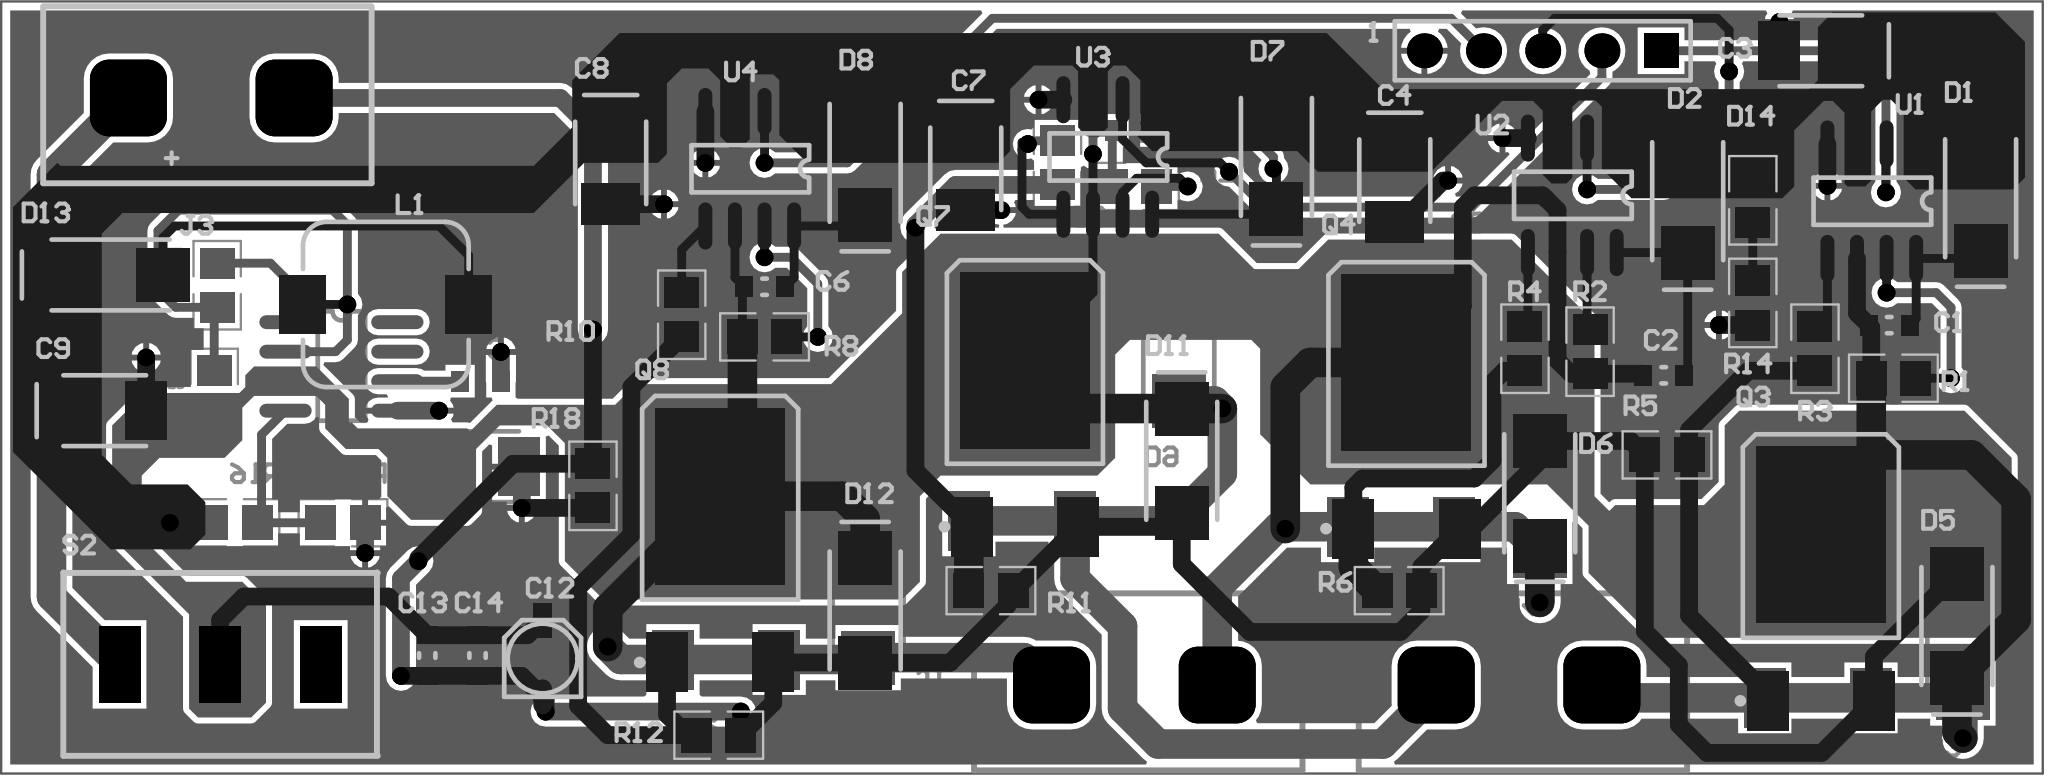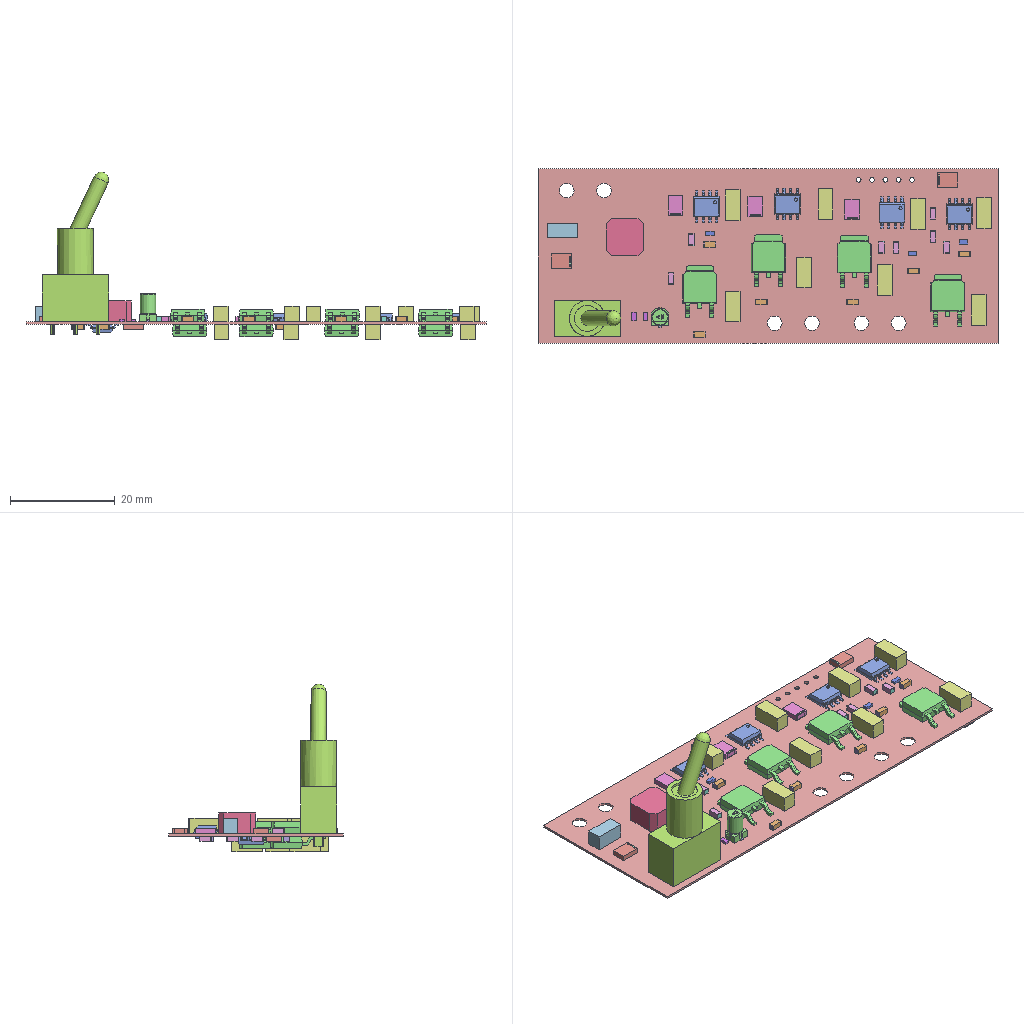Circuit board layout | Altium Designer | box 87.6 x 33.2 x 32 mm
Layer stack:
# Altium Designer layer stack of  (unit mm; dielectric type: 0 none, 1 core, 2 prepreg, 3 surface material)
index,name,kind,layer,copper_thickness_mm,dielectric_type,dielectric_thickness_mm,dielectric_material,dielectric_constant
0,Top Paste,other,,,,,,
1,Top Overlay,other,,,,,,
2,Top Solder,dielectric,,,3,0.0102,Solder Resist,3.5
3,Top Layer,copper,Top Layer,0.0356,,,,
4,Dielectric 1,dielectric,,,0,0.32,FR-4,4.8
5,Bottom Layer,copper,Bottom Layer,0.0356,,,,
6,Bottom Solder,dielectric,,,3,0.0102,Solder Resist,3.5
7,Bottom Overlay,other,,,,,,
8,Bottom Paste,other,,,,,,
# drill layer pairs: low layer,high layer
drill_pair,Top Layer,Bottom Layer
Part placement:
Designator,Comment,Layer,Footprint,Center-X(mm),Center-Y(mm),Rotation
U5,MC34063,BottomLayer,MC34063,33.782,84.455,180
U4,IR2104S,TopLayer,IR2104,51.308,92.964,270
U3,IR2104S,TopLayer,IR2104,66.675,93.472,270
U2,IR2104S,TopLayer,IR2104,86.614,91.821,270
U1,IR2104S,TopLayer,IR2104,99.469,91.567,270
S2,SW-SPST,TopLayer,SWITCH,28.575,71.628,360
R18,Res1,TopLayer,0805,44.577,79.314,270
R17,Res1,BottomLayer,0805,33.848,77.724,360
R16,Res1,BottomLayer,0805,29.21,77.724,360
R15,Res1,BottomLayer,0805,28.448,87.95,270
R14,Res1,TopLayer,0805,94.361,87.188,270
R13,Res1,BottomLayer,0805,28.321,83.312,270
R12,Res1,TopLayer,0805,49.977,68.58,180
R11,Res1,TopLayer,0805,61.661,74.803,180
R10,Res1,TopLayer,0805,48.387,86.68,270
R9,Res1,BottomLayer,0805,64.516,93.218,270
R8,Res1,TopLayer,0805,51.943,85.725,180
R7,Res1,BottomLayer,0805,67.818,92.202,180
R6,Res1,TopLayer,0805,79.182,74.803,180
R5,Res1,TopLayer,0805,90.678,80.645,360
R4,Res1,TopLayer,0805,84.582,85.217,270
R3,Res1,TopLayer,0805,97.028,85.217,270
R2,Res1,TopLayer,0805,87.376,85.09,270
R1,Res1,TopLayer,0805,100.396,83.947,180
Q8,IR7843,TopLayer,LR7843,50.038,75.289,270
Q7,IR7843,TopLayer,LR7843,63.119,81.131,270
Q6,IR7843,BottomLayer,LR7843,50.292,75.416,270
Q5,IR7843,BottomLayer,LR7843,62.992,81.385,270
Q4,IR7843,TopLayer,LR7843,79.496,81.048,270
Q3,IR7843,TopLayer,LR7843,97.282,73.638,270
Q2,IR7843,BottomLayer,LR7843,79.248,81.131,270
Q1,IR7843,BottomLayer,LR7843,97.155,73.765,270
L1,Inductor,TopLayer,L-SMD-7,35.687,87.122,180
J3,Pin2,TopLayer,PCBComponent_1_-_duplicate,28.194,96.012,270
J2,Pin2,BottomLayer,PCBComponent_1_-_duplicate,84.328,70.739,270
J1,Pin2,BottomLayer,PCBComponent_1_-_duplicate,67.818,70.739,270
D14,LED0,TopLayer,0805,94.361,91.606,270
D13,D-Schottky,TopLayer,DIODE-SMA,23.876,88.392,180
D12,D-Schottky,TopLayer,DIODE-SMA,56.261,73.95,90
D11,D-Schottky,TopLayer,DIODE-SMA,69.85,80.391,90
D10,D-Schottky,BottomLayer,DIODE-SMA,56.388,74.168,90
D9,D-Schottky,BottomLayer,DIODE-SMA,69.723,85.217,90
D8,D-Schottky,TopLayer,DIODE-SMA,56.261,93.218,270
D7,D-Schottky,TopLayer,DIODE-SMA,73.914,93.472,270
D6,D-Schottky,TopLayer,DIODE-SMA,85.217,78.994,270
D5,D-Schottky,TopLayer,DIODE-SMA,103.124,73.279,270
D4,D-Schottky,BottomLayer,DIODE-SMA,85.217,78.74,90
D3,D-Schottky,BottomLayer,DIODE-SMA,103.378,72.644,90
D2,D-Schottky,TopLayer,DIODE-SMA,91.567,91.567,270
D1,D-Schottky,TopLayer,DIODE-SMA,104.14,91.694,270
C14,Cap,TopLayer,my0603,39.624,72.009,90
C13,Cap,TopLayer,my0603,37.465,72.009,90
C12,Cap Pol,TopLayer,CM_A(3*5.4),42.418,71.882,90
C11,Cap Pol,BottomLayer,CAP-3528,39.624,80.137,0
C10,Cap,BottomLayer,my0603,39.751,83.82,180
C9,Cap Pol,TopLayer,CAP-3528,23.622,82.55,360
C8,Cap Pol,TopLayer,CAP-3528,45.339,93.218,270
C7,Cap Pol,TopLayer,CAP-3528,60.579,92.964,270
C6,Cap,TopLayer,my0603,51.943,87.884,180
C5,Cap,BottomLayer,my0603,67.818,94.615,180
C4,Cap Pol,TopLayer,CAP-3528,78.994,92.456,270
C3,Cap Pol,TopLayer,CAP-3528,97.282,98.044,180
C2,Cap,TopLayer,my0603,90.537,84.074,180
C1,Cap,TopLayer,my0603,100.217,86.233,180
1,Header 5,TopLayer,HDR1X5,85.344,98.044,180
Pad and via stacks:
# Altium Designer via and pad stacks of  (unit mm). Each distinct definition once, with the count of objects using it.
# via: kind,start_layer,end_layer,hole_mm,diameter_mm,mode(0 simple;1 top-mid-bottom;2 full stack),diameter_per_layer,count,example_net
# pad: kind,layer,hole_mm,hole_type(0 round;1 square;2 slot),plating,top_size,top_shape(1 round;2 rect;3 octagon;9 rounded rect),mid_size,bottom_size,mode,footprint,size_per_layer,count,example
pad,Multi-Layer,1,2,plated,3.3x1.8,2,0x0,3.3x1.8,1,SWITCH,,1,S2.3
pad,Multi-Layer,1,2,plated,3.3x1.8,2,3.3x1.8,3.3x1.8,0,SWITCH,,2,S2.2
pad,Multi-Layer,0.9,0,plated,1.5x1.5,1,1.5x1.5,1.5x1.5,0,HDR1X5,,4,1.5
pad,Multi-Layer,0.9,0,plated,1.5x1.5,2,1.5x1.5,1.5x1.5,0,HDR1X5,,1,1.1
pad,Multi-Layer,2.794,0,plated,3.302x3.302,9,3.302x3.302,3.302x3.302,0,PCBComponent_1 - duplicate,,6,J3.2
pad,Top Layer,0,0,plated,0.6x2.032,1,0.6x2.032,0.6x2.032,0,IR2104,,32,U4.5
pad,Top Layer,0,0,plated,1.5x1.3,2,1.5x1.3,1.5x1.3,0,0805,,26,R14.1
pad,Top Layer,0,0,plated,1.778x2.54,2,1.778x2.54,1.778x2.54,0,LR7843,,8,Q4.1
pad,Top Layer,0,0,plated,5.55x7.6,2,5.55x7.6,5.55x7.6,0,LR7843,,4,Q4.2
pad,Top Layer,0,0,plated,2.3x2.3,2,2.3x2.3,2.3x2.3,0,DIODE-SMA,,18,D13.2
pad,Top Layer,0,0,plated,0.9x0.75,2,0.9x0.75,0.9x0.75,0,my0603,,10,C14.1
pad,Top Layer,0,0,plated,1.5x0.8,1,1.5x0.8,1.5x0.8,0,CM A(3*5.4),,1,C12.2
pad,Top Layer,0,0,plated,1.5x0.8,2,1.5x0.8,1.5x0.8,0,CM A(3*5.4),,1,C12.1
pad,Top Layer,0,0,plated,1.8x2.5,2,1.8x2.5,1.8x2.5,0,CAP-3528,,10,C9.2
pad,Top Layer,0,0,plated,2.5x2,2,2.5x2,2.5x2,0,L-SMD-7,,2,L1.1
pad,Bottom Layer,0,0,plated,1.778x2.54,2,1.778x2.54,1.778x2.54,0,LR7843,,8,Q6.1
pad,Bottom Layer,0,0,plated,5.55x7.6,2,5.55x7.6,5.55x7.6,0,LR7843,,4,Q6.2
pad,Bottom Layer,0,0,plated,2.3x2.3,2,2.3x2.3,2.3x2.3,0,DIODE-SMA,,8,D10.2
pad,Bottom Layer,0,0,plated,0.6x2.25,1,0.6x2.25,0.6x2.25,0,MC34063,,8,U5.5
pad,Bottom Layer,0,0,plated,1.5x1.3,2,1.5x1.3,1.5x1.3,0,0805,,12,R15.1
pad,Bottom Layer,0,0,plated,0.9x0.75,2,0.9x0.75,0.9x0.75,0,my0603,,4,C10.1
pad,Bottom Layer,0,0,plated,1.8x2.5,2,1.8x2.5,1.8x2.5,0,CAP-3528,,2,C11.2
via,Top Layer,Bottom Layer,0.381,0.762,0,,40,+12
Copper pours:
name,layer,net,type(0 solid;1 hatched;2 none)
D,Bottom Layer,GND,0
Design rules, without the lines most boards share:
# Altium Designer design rules of  (exported by Altium Designer, unit mm)
# columns: name | kind | enabled | priority | scope1 | scope2 | descriptor | typed fields (field=value)
NetAntennae | 56 | enabled | 1 | All | All | Net Antennae (Tolerance=0mm) (All) |
SilkToSilkClearance | 55 | enabled | 1 | All | All | Silk to Silk (Clearance=0mm) (All),(All) |
SilkToSolderMaskClearance | 54 | enabled | 1 | IsPad | All | Silk To Solder Mask (Clearance=0mm) (IsPad),(All) |
MinimumSolderMaskSliver | 53 | enabled | 1 | All | All | Minimum Solder Mask Sliver (Gap=0mm) (All),(All) |
HoleToHoleClearance | 52 | enabled | 1 | All | All | Hole To Hole Clearance (Gap=0.254mm) (All),(All) | gap=0.254
DiffPairsRouting | 51 | enabled | 1 | All | All | Differential Pairs Uncoupled Length using the Gap Constraints (Min=0.254mm) (Max=0.254mm) (Prefered=0.254mm)  and Width Constraints (Min=0.381mm) (Max=0.381mm) (Prefered=0.381mm) (All) |
HoleSize | 42 | enabled | 1 | All | All | Hole Size Constraint (Min=0.025mm) (Max=254mm) (All) |
Height | 50 | enabled | 1 | All | All | Height Constraint (Min=0mm) (Max=100mm) (Prefered=12.7mm) (All) | min_height=0 max_height=100
ComponentClearance | 24 | enabled | 1 | All | All | Component Clearance Constraint ( Horizontal Gap = 0.254mm, Vertical Gap = 0.254mm ) (All),(All)  | gap=0.254
SolderMaskExpansion | 13 | enabled | 1 | All | All | Solder Mask Expansion (Expansion =0.102mm) (All) | expansion=0.1016
PasteMaskExpansion | 14 | enabled | 1 | All | All | Paste Mask Expansion (Expansion =0mm) (All) | expansion=0
RoutingVias | 11 | enabled | 1 | All | All | Routing Via (MinHoleWidth=0.711mm) (MaxHoleWidth=0.711mm) (PreferredHoleWidth=0.711mm) (MinWidth=1.27mm) (MaxWidth=1.27mm) (PreferedWidth=1.27mm) (All) | via_min_hole=0.7112 via_max_hole=0.7112 via_preferred_diameter=1.27 via_preferred_hole=0.7112
RoutingCorners | 10 | enabled | 1 | All | All | Routing Corners (Style=45-Degree) (Min Setback=2.54mm) (Max Setback=2.54mm) (All) |
Width | 2 | enabled | 1 | All | All | Width Constraint (Min=0.254mm) (Max=2.032mm) (Preferred=0.254mm) (All) |
PolygonConnect | 20 | enabled | 1 | All | All | Polygon Connect Rule(Relief Connect )(Conductor Width=0.254mm) (Relief Angle=90 Angle) (Entries=4) (Air Gap Width=0.254mm) (All),(All) | connect_style(0=relief,1=direct,2=none)=0 relief_conductor_width=0.254 relief_entries=4
PlaneClearance | 12 | enabled | 1 | All | All | Power Plane Clearance (Clearance =0.508mm) (All) | clearance=0.508
PlaneConnect | 6 | enabled | 1 | All | All | Power Plane Connect Rule(Relief Connect )(Expansion=0.508mm) (Conductor Width=0.254mm) (Air Gap=0.254mm) (Entries=4) (All) | relief_conductor_width=0.254 relief_entries=4 relief_expansion=0.508
Clearance | 0 | enabled | 1 | All | All | Clearance Constraint (Gap=0.254mm) (All),(All) | gap=0.254